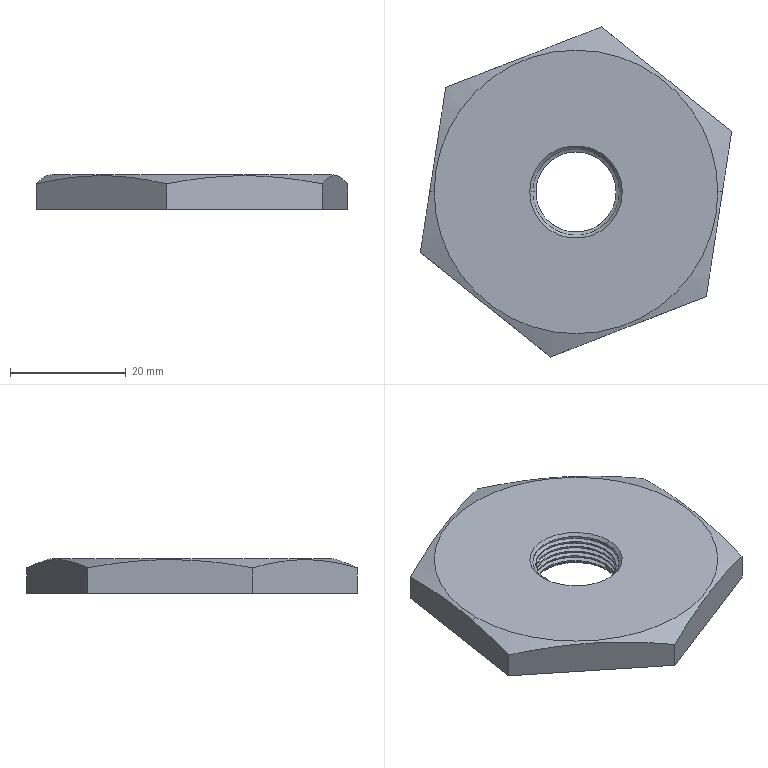Part | STEP file | Adjusting nut 2 | 1 solid | 28 faces | box 53.803 x 57.066 x 6 mm | volume 11857 mm3 | cylinder 11 | plane 10 | cone 4 | spline 3 | commonest cylinder face diameters 15 x11